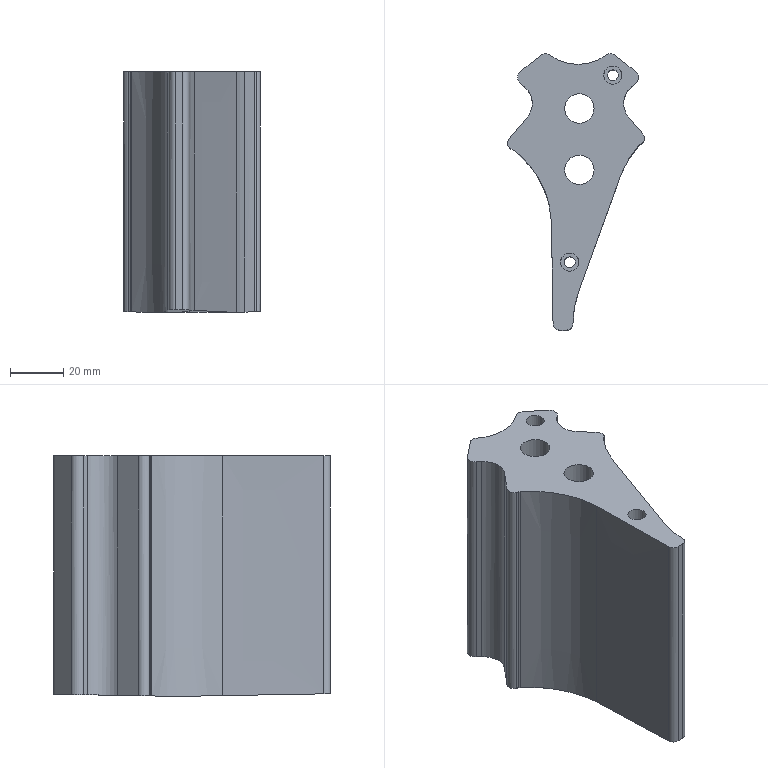Part | STEP file | gslz 2016.10.28-10_id3190_x_t | 1 solid | 44 faces | box 51.195 x 103.6 x 90 mm | volume 199398 mm3 | cylinder 21 | plane 16 | other 7 | commonest cylinder face diameters 5 x8 4.1 x2 6 x2 6.8 x2 11 x2 16 x2